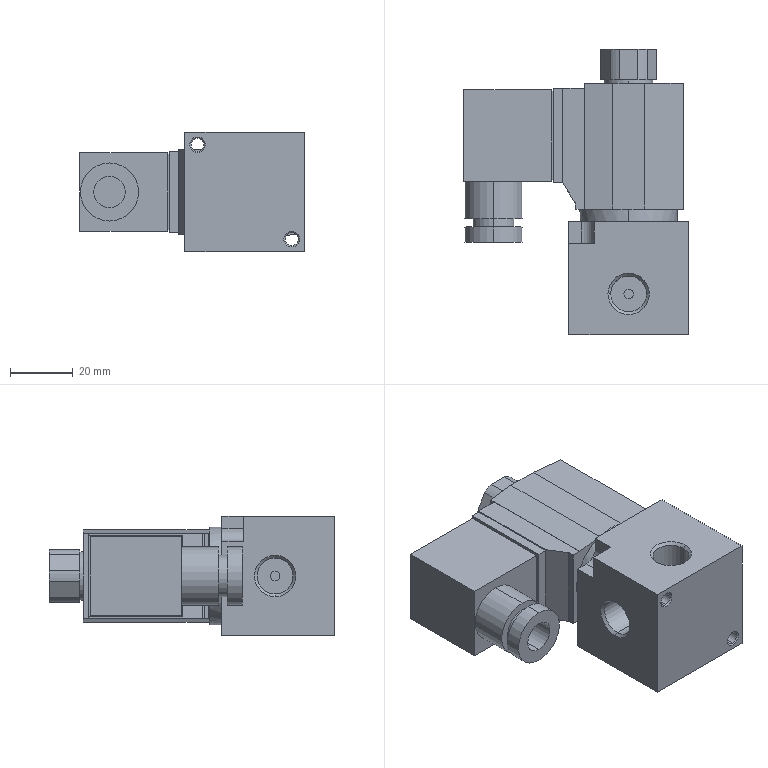Part | STEP file | 3V308NCB | 1 solid | 118 faces | box 71.5 x 90.9 x 38 mm | volume 121350 mm3 | plane 66 | cylinder 42 | cone 10 | commonest cylinder face diameters 3 x6 11.445 x6 18 x6 4.134 x4 4.2 x4 18.5 x4